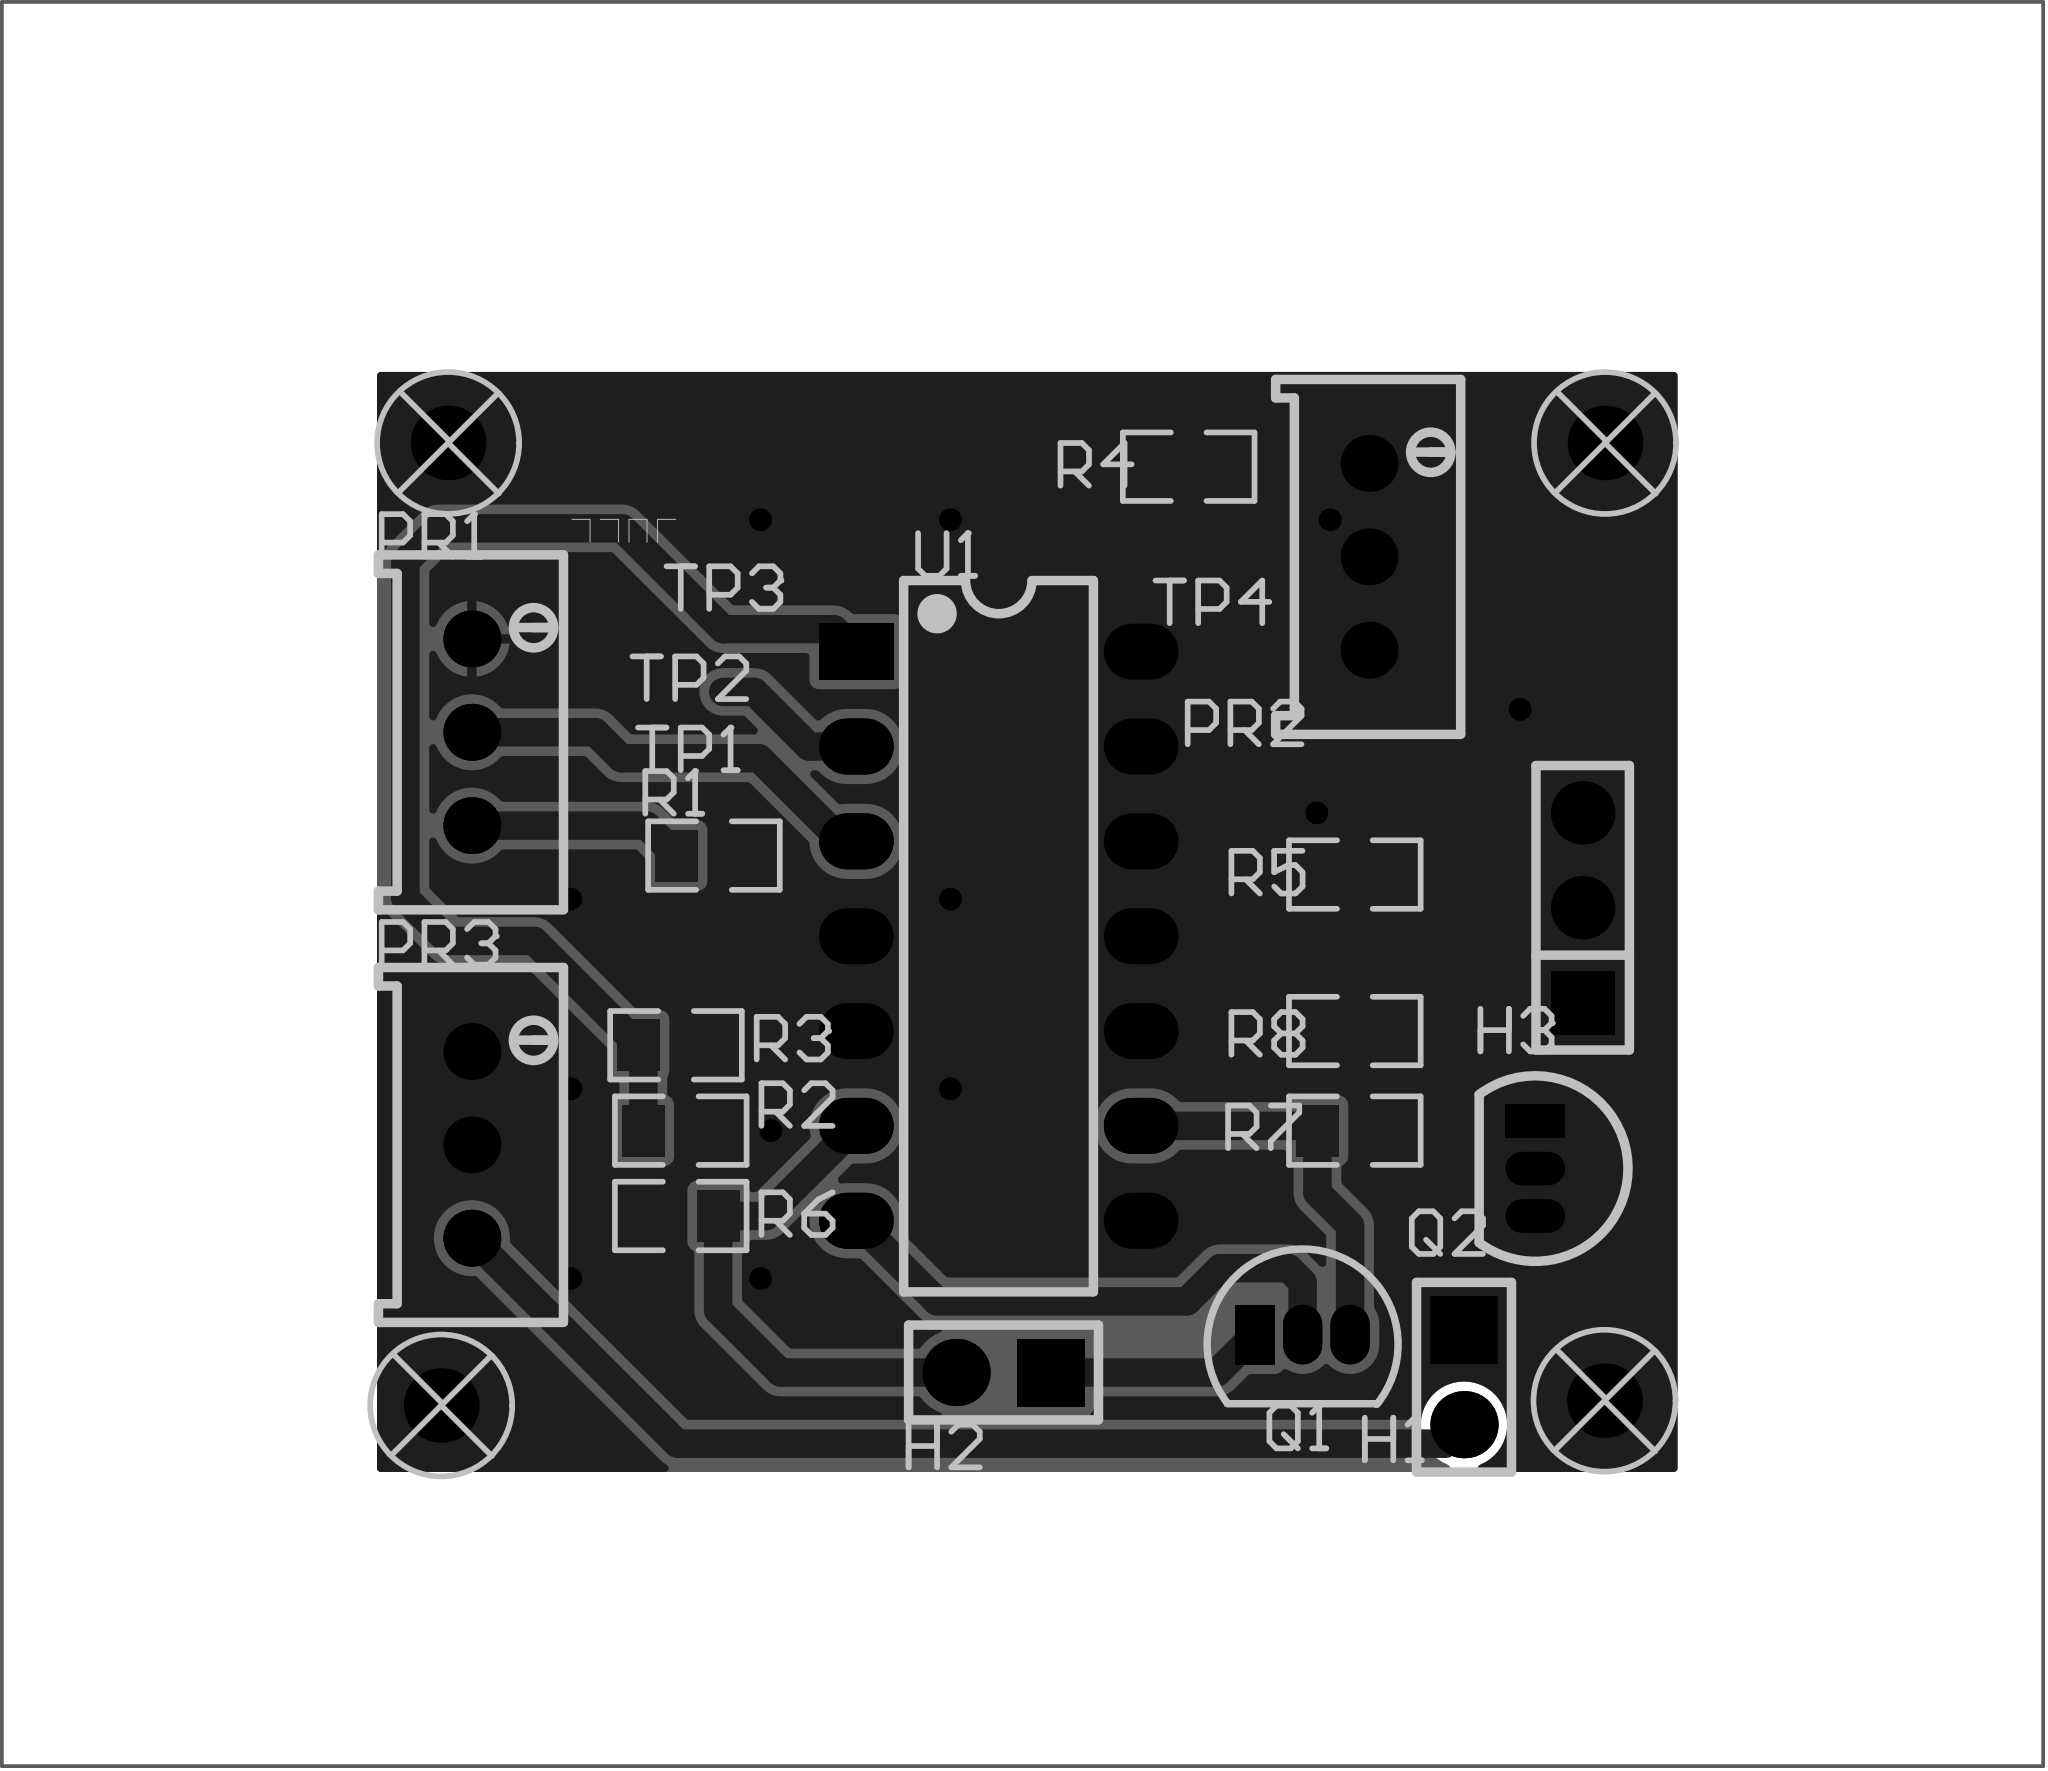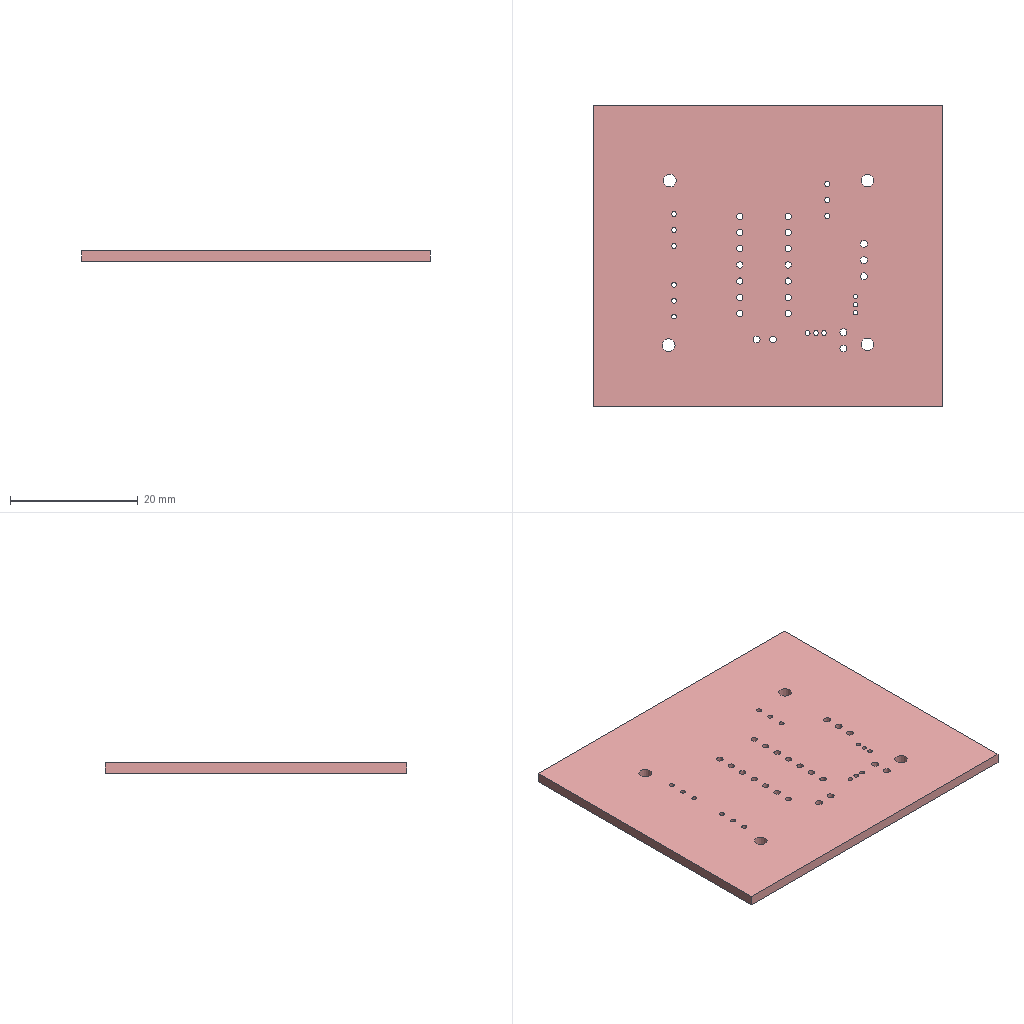Circuit board layout | Altium Designer | box 54.6 x 47.2 x 1.6 mm
Layer stack:
# Altium Designer layer stack of  (unit mm; dielectric type: 0 none, 1 core, 2 prepreg, 3 surface material)
index,name,kind,layer,copper_thickness_mm,dielectric_type,dielectric_thickness_mm,dielectric_material,dielectric_constant
0,Top Paste Mask Layer,other,,,,,,
1,Top Silkscreen Layer,other,,,,,,
2,Top Solder Mask Layer,dielectric,,,3,0.01,,3.3
3,Top Layer,copper,Top Layer,0.035,,,,
4,Dielectric1,dielectric,,,3,1.51,FR4,4.5
5,Bottom Layer,copper,Bottom Layer,0.035,,,,
6,Bottom Solder Mask Layer,dielectric,,,3,0.01,,3.3
7,Bottom Silkscreen Layer,other,,,,,,
8,Bottom Paste Mask Layer,other,,,,,,
# drill layer pairs: low layer,high layer
drill_pair,Top Layer,Bottom Layer
Part placement:
Designator,Comment,Layer,Footprint,Center-X(mm),Center-Y(mm),Rotation
H1,,TopLayer,HDR-TH_2P-P2.54-V-M-1,108.966,80.264,270
H2,,TopLayer,HDR-TH_2P-P2.54-V-M-1,96.647,80.391,180
PR1,20kΩ,TopLayer,R_3296,82.423,97.536,270
PR2,10kΩ,TopLayer,R_3296,106.426,102.235,270
PR3,250,TopLayer,R_3296,82.423,86.487,270
Q1,2N2222A,TopLayer,TO-92-3_L5.1-W4.1-P1.27-L-1,104.648,81.407,0
Q2,2SA1015(RANGE:200-400),TopLayer,TO-92-3_L4.9-W3.7-P1.27-L,110.871,85.852,270
R1,40K,TopLayer,R0805,88.9,94.234,0
R2,1K,TopLayer,R0805,88.011,86.868,0
R3,1K,TopLayer,R0805,87.884,89.154,180
R4,1K,TopLayer,R0805,101.6,104.648,180
R5,10K,TopLayer,R0805,106.045,93.726,0
R6,249,TopLayer,R0805,88.011,84.582,180
R7,804,TopLayer,R0805,106.045,86.868,180
R8,804,TopLayer,R0805,106.045,89.535,180
TP1,,TopLayer,Test-Point-0.5mm,89.146,96.84,180
TP2,,TopLayer,Test-Point-0.5mm,89.146,98.618,90
TP3,,TopLayer,Test-Point-0.5mm,89.146,100.297,90
TP4,,TopLayer,Test-Point-0.5mm,101.659,102.174,0
U1,LM324N196,TopLayer,PDIP-14_L19.3-W6.5-P2.54-LS7.6-BL,96.52,92.075,270
H3,,TopLayer,HDR-TH_3P-P2.54-V-M,112.141,92.837,90
SCREW1,,TopLayer,M2螺丝,81.603,79.508,0
SCREW2,,TopLayer,M2螺丝,112.725,79.635,0
SCREW3,,TopLayer,M2螺丝,81.788,105.283,0
SCREW4,,TopLayer,M2螺丝,112.739,105.282,0
Pad and via stacks:
# Altium Designer via and pad stacks of  (unit mm). Each distinct definition once, with the count of objects using it.
# via: kind,start_layer,end_layer,hole_mm,diameter_mm,mode(0 simple;1 top-mid-bottom;2 full stack),diameter_per_layer,count,example_net
# pad: kind,layer,hole_mm,hole_type(0 round;1 square;2 slot),plating,top_size,top_shape(1 round;2 rect;3 octagon;9 rounded rect),mid_size,bottom_size,mode,footprint,size_per_layer,count,example
pad,Multi-Layer,1.1,0,plated,1.8x1.8,1,1.8x1.8,1.8x1.8,0,HDR-TH_2P-P2.54-V-M-1,,2,H1.2
pad,Multi-Layer,1.1,0,plated,1.8x1.8,2,1.8x1.8,1.8x1.8,0,HDR-TH_2P-P2.54-V-M-1,,2,H1.1
pad,Multi-Layer,0.762,0,plated,1.524x1.524,1,1.524x1.524,1.524x1.524,0,R_3296,,9,PR1.2
pad,Multi-Layer,0.75,0,plated,1.05x1.6,2,1.05x1.6,1.05x1.6,0,TO-92-3_L5.1-W4.1-P1.27-L-1,,1,Q1.1
pad,Multi-Layer,0.75,0,plated,1.05x1.6,1,1.05x1.6,1.05x1.6,0,TO-92-3_L5.1-W4.1-P1.27-L-1,,2,Q1.2
pad,Multi-Layer,0.7,0,plated,0.9x1.6,1,0.9x1.6,0.9x1.6,0,TO-92-3_L4.9-W3.7-P1.27-L,,2,Q2.3
pad,Multi-Layer,0.7,0,plated,0.9x1.6,2,0.9x1.6,0.9x1.6,0,TO-92-3_L4.9-W3.7-P1.27-L,,1,Q2.1
pad,Multi-Layer,1,0,plated,1.5x2,1,1.5x2,1.5x2,0,PDIP-14_L19.3-W6.5-P2.54-LS7.6-BL,,13,U1.8
pad,Multi-Layer,1,0,plated,1.5x2,2,1.5x2,1.5x2,0,PDIP-14_L19.3-W6.5-P2.54-LS7.6-BL,,1,U1.1
pad,Multi-Layer,1.1,0,plated,1.7x1.7,2,1.7x1.7,1.7x1.7,0,HDR-TH_3P-P2.54-V-M,,1,H3.1
pad,Multi-Layer,1.1,0,plated,1.7x1.7,1,1.7x1.7,1.7x1.7,0,HDR-TH_3P-P2.54-V-M,,2,H3.2
pad,Multi-Layer,2,0,plated,2x2,1,2x2,2x2,0,M2\u00C2\u00DD\u00CB\u00BF,,4,SCREW1.1
pad,Top Layer,0,0,plated,1.133x1.377,2,1.133x1.377,1.133x1.377,0,R0805,,16,R1.2
pad,Top Layer,0,0,plated,0.5x0.5,1,0.5x0.5,0.5x0.5,0,Test-Point-0.5mm,,4,TP1.1
via,Top Layer,Bottom Layer,0.3048,0.61,0,,12,$1N8
Copper pours:
name,layer,net,type(0 solid;1 hatched;2 none)
Top Layer-GND,Top Layer,GND,0
Bottom Layer-GND,Bottom Layer,GND,0